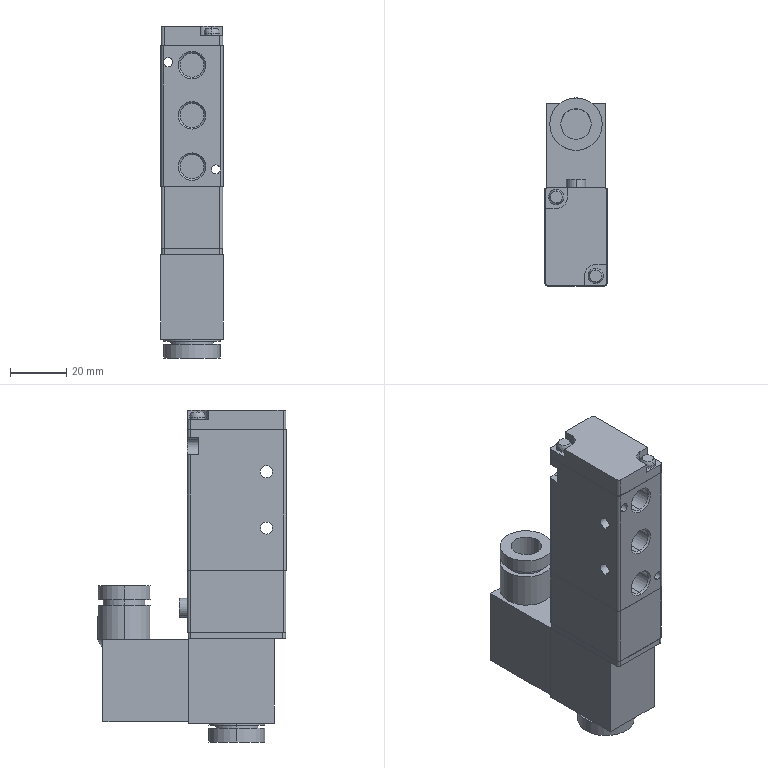Part | STEP file | 4V21006B | 1 solid | 136 faces | box 22 x 66.8 x 117.8 mm | volume 101337 mm3 | plane 61 | cylinder 60 | cone 11 | sphere 4 | commonest cylinder face diameters 2 x18 8.566 x10 3.2 x4 4.3 x4 5.4 x4 15 x4